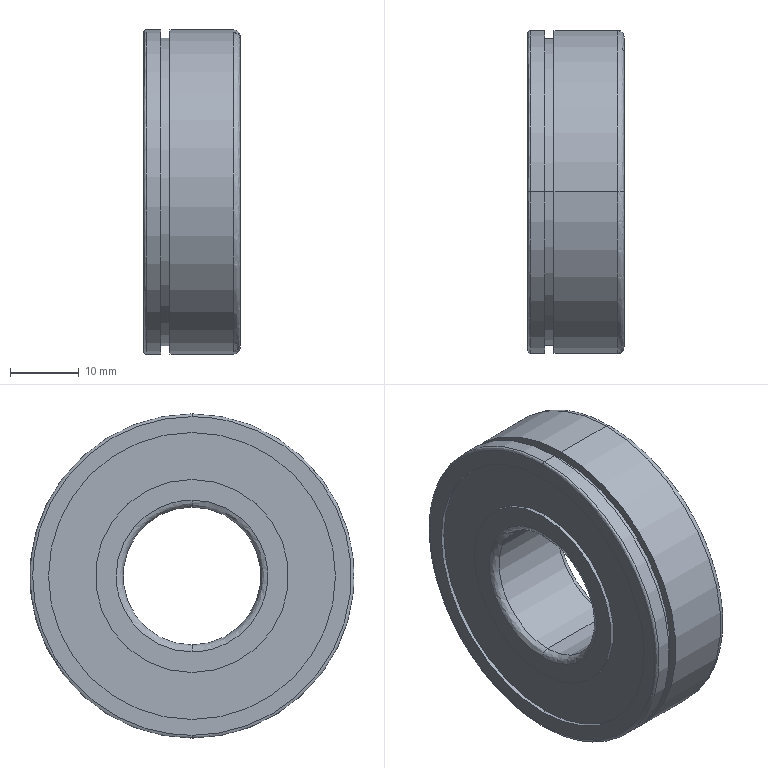Part | STEP file | 0229_Z_B6204ZZNR_1 | 1 solid | 32 faces | box 14 x 47 x 47 mm | volume 18805 mm3 | cylinder 16 | spline 8 | plane 8 | commonest cylinder face diameters 28 x4 41.6 x4 47 x4 20 x2 44.6 x2